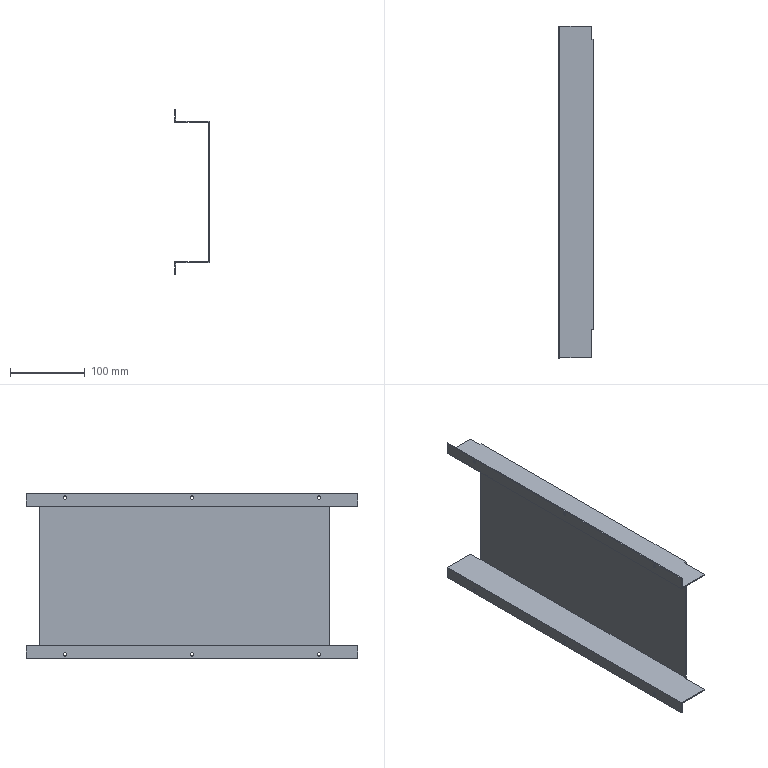Part | SolidWorks | features BaseBody 1 | 1 solid | 34 faces | box 46.5 x 444 x 220 mm | volume 190195 mm3 | plane 22 | cylinder 12 | commonest cylinder face diameters 4.4 x12
STEP:
#1=CARTESIAN_POINT('',(900.946,-4005.973,1042.771));
#2=VERTEX_POINT('',#1);
#3=CARTESIAN_POINT('',(900.946,-4005.973,1047.171));
#4=VERTEX_POINT('',#3);
#5=CARTESIAN_POINT('',(900.946,-4005.973,1044.971));
#6=DIRECTION('',(-1.,0.,0.));
#7=DIRECTION('',(0.,0.,1.));
#8=AXIS2_PLACEMENT_3D('',#5,#6,#7);
#9=CIRCLE('',#8,2.2);
#10=EDGE_CURVE('',#2,#4,#9,.T.);
#11=ORIENTED_EDGE('',*,*,#10,.F.);
#12=CARTESIAN_POINT('',(899.446,-4005.973,1042.771));
#13=VERTEX_POINT('',#12);
#14=CARTESIAN_POINT('',(897.509,-4005.973,1042.771));
#15=DIRECTION('',(-1.,0.,0.));
#16=VECTOR('',#15,1000.);
#17=LINE('',#14,#16);
#18=EDGE_CURVE('',#2,#13,#17,.T.);
#19=ORIENTED_EDGE('',*,*,#18,.T.);
#20=CARTESIAN_POINT('',(899.446,-4005.973,1047.171));
#21=VERTEX_POINT('',#20);
#22=CARTESIAN_POINT('',(899.446,-4005.973,1044.971));
#23=DIRECTION('',(1.,0.,0.));
#24=DIRECTION('',(0.,0.,1.));
#25=AXIS2_PLACEMENT_3D('',#22,#23,#24);
#26=CIRCLE('',#25,2.2);
#27=EDGE_CURVE('',#21,#13,#26,.T.);
#28=ORIENTED_EDGE('',*,*,#27,.F.);
#29=CARTESIAN_POINT('',(897.509,-4005.973,1047.171));
#30=DIRECTION('',(-1.,0.,0.));
#31=VECTOR('',#30,1000.);
#32=LINE('',#29,#31);
#33=EDGE_CURVE('',#4,#21,#32,.T.);
#34=ORIENTED_EDGE('',*,*,#33,.F.);
#35=EDGE_LOOP('',(#11,#19,#28,#34));
#36=FACE_OUTER_BOUND('',#35,.T.);
#37=CARTESIAN_POINT('',(897.509,-4005.973,1044.971));
#38=DIRECTION('',(-1.,0.,0.));
#39=DIRECTION('',(0.,0.,1.));
#40=AXIS2_PLACEMENT_3D('',#37,#38,#39);
#41=CYLINDRICAL_SURFACE('',#40,2.2);
#42=ADVANCED_FACE('',(#36),#41,.F.);
#43=CARTESIAN_POINT('',(900.946,-4345.973,1042.771));
#44=VERTEX_POINT('',#43);
#45=CARTESIAN_POINT('',(900.946,-4345.973,1047.171));
#46=VERTEX_POINT('',#45);
#47=CARTESIAN_POINT('',(900.946,-4345.973,1044.971));
#48=DIRECTION('',(-1.,0.,0.));
#49=DIRECTION('',(0.,0.,1.));
#50=AXIS2_PLACEMENT_3D('',#47,#48,#49);
#51=CIRCLE('',#50,2.2);
#52=EDGE_CURVE('',#44,#46,#51,.T.);
#53=ORIENTED_EDGE('',*,*,#52,.F.);
#54=CARTESIAN_POINT('',(899.446,-4345.973,1042.771));
#55=VERTEX_POINT('',#54);
#56=CARTESIAN_POINT('',(897.509,-4345.973,1042.771));
#57=DIRECTION('',(-1.,0.,0.));
#58=VECTOR('',#57,1000.);
#59=LINE('',#56,#58);
#60=EDGE_CURVE('',#44,#55,#59,.T.);
#61=ORIENTED_EDGE('',*,*,#60,.T.);
#62=CARTESIAN_POINT('',(899.446,-4345.973,1047.171));
#63=VERTEX_POINT('',#62);
#64=CARTESIAN_POINT('',(899.446,-4345.973,1044.971));
#65=DIRECTION('',(1.,0.,0.));
#66=DIRECTION('',(0.,0.,1.));
#67=AXIS2_PLACEMENT_3D('',#64,#65,#66);
#68=CIRCLE('',#67,2.2);
#69=EDGE_CURVE('',#63,#55,#68,.T.);
#70=ORIENTED_EDGE('',*,*,#69,.F.);
#71=CARTESIAN_POINT('',(897.509,-4345.973,1047.171));
#72=DIRECTION('',(-1.,0.,0.));
#73=VECTOR('',#72,1000.);
#74=LINE('',#71,#73);
#75=EDGE_CURVE('',#46,#63,#74,.T.);
#76=ORIENTED_EDGE('',*,*,#75,.F.);
#77=EDGE_LOOP('',(#53,#61,#70,#76));
#78=FACE_OUTER_BOUND('',#77,.T.);
#79=CARTESIAN_POINT('',(897.509,-4345.973,1044.971));
#80=DIRECTION('',(-1.,0.,0.));
#81=DIRECTION('',(0.,0.,1.));
#82=AXIS2_PLACEMENT_3D('',#79,#80,#81);
#83=CYLINDRICAL_SURFACE('',#82,2.2);
#84=ADVANCED_FACE('',(#78),#83,.F.);
#85=CARTESIAN_POINT('',(900.946,-4175.973,1042.771));
#86=VERTEX_POINT('',#85);
#87=CARTESIAN_POINT('',(900.946,-4175.973,1047.171));
#88=VERTEX_POINT('',#87);
#89=CARTESIAN_POINT('',(900.946,-4175.973,1044.971));
#90=DIRECTION('',(-1.,0.,0.));
#91=DIRECTION('',(0.,0.,1.));
#92=AXIS2_PLACEMENT_3D('',#89,#90,#91);
#93=CIRCLE('',#92,2.2);
#94=EDGE_CURVE('',#86,#88,#93,.T.);
#95=ORIENTED_EDGE('',*,*,#94,.F.);
#96=CARTESIAN_POINT('',(899.446,-4175.973,1042.771));
#97=VERTEX_POINT('',#96);
#98=CARTESIAN_POINT('',(897.509,-4175.973,1042.771));
#99=DIRECTION('',(-1.,0.,0.));
#100=VECTOR('',#99,1000.);
#101=LINE('',#98,#100);
#102=EDGE_CURVE('',#86,#97,#101,.T.);
#103=ORIENTED_EDGE('',*,*,#102,.T.);
#104=CARTESIAN_POINT('',(899.446,-4175.973,1047.171));
#105=VERTEX_POINT('',#104);
#106=CARTESIAN_POINT('',(899.446,-4175.973,1044.971));
#107=DIRECTION('',(1.,0.,0.));
#108=DIRECTION('',(0.,0.,1.));
#109=AXIS2_PLACEMENT_3D('',#106,#107,#108);
#110=CIRCLE('',#109,2.2);
#111=EDGE_CURVE('',#105,#97,#110,.T.);
#112=ORIENTED_EDGE('',*,*,#111,.F.);
#113=CARTESIAN_POINT('',(897.509,-4175.973,1047.171));
#114=DIRECTION('',(-1.,0.,0.));
#115=VECTOR('',#114,1000.);
#116=LINE('',#113,#115);
#117=EDGE_CURVE('',#88,#105,#116,.T.);
#118=ORIENTED_EDGE('',*,*,#117,.F.);
#119=EDGE_LOOP('',(#95,#103,#112,#118));
#120=FACE_OUTER_BOUND('',#119,.T.);
#121=CARTESIAN_POINT('',(897.509,-4175.973,1044.971));
#122=DIRECTION('',(-1.,0.,0.));
#123=DIRECTION('',(0.,0.,1.));
#124=AXIS2_PLACEMENT_3D('',#121,#122,#123);
#125=CYLINDRICAL_SURFACE('',#124,2.2);
#126=ADVANCED_FACE('',(#120),#125,.F.);
#127=CARTESIAN_POINT('',(899.446,-4175.973,837.171));
#128=VERTEX_POINT('',#127);
#129=CARTESIAN_POINT('',(899.446,-4175.973,832.771));
#130=VERTEX_POINT('',#129);
#131=CARTESIAN_POINT('',(899.446,-4175.973,834.971));
#132=DIRECTION('',(1.,0.,0.));
#133=DIRECTION('',(0.,0.,-1.));
#134=AXIS2_PLACEMENT_3D('',#131,#132,#133);
#135=CIRCLE('',#134,2.2);
#136=EDGE_CURVE('',#128,#130,#135,.T.);
#137=ORIENTED_EDGE('',*,*,#136,.F.);
#138=CARTESIAN_POINT('',(900.946,-4175.973,837.171));
#139=VERTEX_POINT('',#138);
#140=CARTESIAN_POINT('',(897.509,-4175.973,837.171));
#141=DIRECTION('',(1.,0.,0.));
#142=VECTOR('',#141,1000.);
#143=LINE('',#140,#142);
#144=EDGE_CURVE('',#128,#139,#143,.T.);
#145=ORIENTED_EDGE('',*,*,#144,.T.);
#146=CARTESIAN_POINT('',(900.946,-4175.973,832.771));
#147=VERTEX_POINT('',#146);
#148=CARTESIAN_POINT('',(900.946,-4175.973,834.971));
#149=DIRECTION('',(-1.,0.,0.));
#150=DIRECTION('',(0.,0.,-1.));
#151=AXIS2_PLACEMENT_3D('',#148,#149,#150);
#152=CIRCLE('',#151,2.2);
#153=EDGE_CURVE('',#147,#139,#152,.T.);
#154=ORIENTED_EDGE('',*,*,#153,.F.);
#155=CARTESIAN_POINT('',(897.509,-4175.973,832.771));
#156=DIRECTION('',(1.,0.,0.));
#157=VECTOR('',#156,1000.);
#158=LINE('',#155,#157);
#159=EDGE_CURVE('',#130,#147,#158,.T.);
#160=ORIENTED_EDGE('',*,*,#159,.F.);
#161=EDGE_LOOP('',(#137,#145,#154,#160));
#162=FACE_OUTER_BOUND('',#161,.T.);
#163=CARTESIAN_POINT('',(897.509,-4175.973,834.971));
#164=DIRECTION('',(1.,0.,0.));
#165=DIRECTION('',(0.,0.,-1.));
#166=AXIS2_PLACEMENT_3D('',#163,#164,#165);
#167=CYLINDRICAL_SURFACE('',#166,2.2);
#168=ADVANCED_FACE('',(#162),#167,.F.);
#169=CARTESIAN_POINT('',(899.446,-4345.973,837.171));
#170=VERTEX_POINT('',#169);
#171=CARTESIAN_POINT('',(899.446,-4345.973,832.771));
#172=VERTEX_POINT('',#171);
#173=CARTESIAN_POINT('',(899.446,-4345.973,834.971));
#174=DIRECTION('',(1.,0.,0.));
#175=DIRECTION('',(0.,0.,-1.));
#176=AXIS2_PLACEMENT_3D('',#173,#174,#175);
#177=CIRCLE('',#176,2.2);
#178=EDGE_CURVE('',#170,#172,#177,.T.);
#179=ORIENTED_EDGE('',*,*,#178,.F.);
#180=CARTESIAN_POINT('',(900.946,-4345.973,837.171));
#181=VERTEX_POINT('',#180);
#182=CARTESIAN_POINT('',(897.509,-4345.973,837.171));
#183=DIRECTION('',(1.,0.,0.));
#184=VECTOR('',#183,1000.);
#185=LINE('',#182,#184);
#186=EDGE_CURVE('',#170,#181,#185,.T.);
#187=ORIENTED_EDGE('',*,*,#186,.T.);
#188=CARTESIAN_POINT('',(900.946,-4345.973,832.771));
#189=VERTEX_POINT('',#188);
#190=CARTESIAN_POINT('',(900.946,-4345.973,834.971));
#191=DIRECTION('',(-1.,0.,0.));
#192=DIRECTION('',(0.,0.,-1.));
#193=AXIS2_PLACEMENT_3D('',#190,#191,#192);
#194=CIRCLE('',#193,2.2);
#195=EDGE_CURVE('',#189,#181,#194,.T.);
#196=ORIENTED_EDGE('',*,*,#195,.F.);
#197=CARTESIAN_POINT('',(897.509,-4345.973,832.771));
#198=DIRECTION('',(1.,0.,0.));
#199=VECTOR('',#198,1000.);
#200=LINE('',#197,#199);
#201=EDGE_CURVE('',#172,#189,#200,.T.);
#202=ORIENTED_EDGE('',*,*,#201,.F.);
#203=EDGE_LOOP('',(#179,#187,#196,#202));
#204=FACE_OUTER_BOUND('',#203,.T.);
#205=CARTESIAN_POINT('',(897.509,-4345.973,834.971));
#206=DIRECTION('',(1.,0.,0.));
#207=DIRECTION('',(0.,0.,-1.));
#208=AXIS2_PLACEMENT_3D('',#205,#206,#207);
#209=CYLINDRICAL_SURFACE('',#208,2.2);
#210=ADVANCED_FACE('',(#204),#209,.F.);
#211=CARTESIAN_POINT('',(899.446,-4005.973,837.171));
#212=VERTEX_POINT('',#211);
#213=CARTESIAN_POINT('',(899.446,-4005.973,832.771));
#214=VERTEX_POINT('',#213);
#215=CARTESIAN_POINT('',(899.446,-4005.973,834.971));
#216=DIRECTION('',(1.,0.,0.));
#217=DIRECTION('',(0.,0.,-1.));
#218=AXIS2_PLACEMENT_3D('',#215,#216,#217);
#219=CIRCLE('',#218,2.2);
#220=EDGE_CURVE('',#212,#214,#219,.T.);
#221=ORIENTED_EDGE('',*,*,#220,.F.);
#222=CARTESIAN_POINT('',(900.946,-4005.973,837.171));
#223=VERTEX_POINT('',#222);
#224=CARTESIAN_POINT('',(897.509,-4005.973,837.171));
#225=DIRECTION('',(1.,0.,0.));
#226=VECTOR('',#225,1000.);
#227=LINE('',#224,#226);
#228=EDGE_CURVE('',#212,#223,#227,.T.);
#229=ORIENTED_EDGE('',*,*,#228,.T.);
#230=CARTESIAN_POINT('',(900.946,-4005.973,832.771));
#231=VERTEX_POINT('',#230);
#232=CARTESIAN_POINT('',(900.946,-4005.973,834.971));
#233=DIRECTION('',(-1.,0.,0.));
#234=DIRECTION('',(0.,0.,-1.));
#235=AXIS2_PLACEMENT_3D('',#232,#233,#234);
#236=CIRCLE('',#235,2.2);
#237=EDGE_CURVE('',#231,#223,#236,.T.);
#238=ORIENTED_EDGE('',*,*,#237,.F.);
#239=CARTESIAN_POINT('',(897.509,-4005.973,832.771));
#240=DIRECTION('',(1.,0.,0.));
#241=VECTOR('',#240,1000.);
#242=LINE('',#239,#241);
#243=EDGE_CURVE('',#214,#231,#242,.T.);
#244=ORIENTED_EDGE('',*,*,#243,.F.);
#245=EDGE_LOOP('',(#221,#229,#238,#244));
#246=FACE_OUTER_BOUND('',#245,.T.);
#247=CARTESIAN_POINT('',(897.509,-4005.973,834.971));
#248=DIRECTION('',(1.,0.,0.));
#249=DIRECTION('',(0.,0.,-1.));
#250=AXIS2_PLACEMENT_3D('',#247,#248,#249);
#251=CYLINDRICAL_SURFACE('',#250,2.2);
#252=ADVANCED_FACE('',(#246),#251,.F.);
#253=CARTESIAN_POINT('',(945.946,-3971.973,844.971));
#254=VERTEX_POINT('',#253);
#255=CARTESIAN_POINT('',(945.946,-3971.973,1034.971));
#256=VERTEX_POINT('',#255);
#257=CARTESIAN_POINT('',(945.946,-3971.973,1014.971));
#258=DIRECTION('',(0.,0.,1.));
#259=VECTOR('',#258,1000.);
#260=LINE('',#257,#259);
#261=EDGE_CURVE('',#254,#256,#260,.T.);
#262=ORIENTED_EDGE('',*,*,#261,.T.);
#263=CARTESIAN_POINT('',(945.946,-4359.973,1034.971));
#264=VERTEX_POINT('',#263);
#265=CARTESIAN_POINT('',(945.946,-3953.973,1034.971));
#266=DIRECTION('',(0.,-1.,0.));
#267=VECTOR('',#266,1000.);
#268=LINE('',#265,#267);
#269=EDGE_CURVE('',#256,#264,#268,.T.);
#270=ORIENTED_EDGE('',*,*,#269,.T.);
#271=CARTESIAN_POINT('',(945.946,-4359.973,844.971));
#272=VERTEX_POINT('',#271);
#273=CARTESIAN_POINT('',(945.946,-4359.973,1014.971));
#274=DIRECTION('',(0.,0.,-1.));
#275=VECTOR('',#274,1000.);
#276=LINE('',#273,#275);
#277=EDGE_CURVE('',#264,#272,#276,.T.);
#278=ORIENTED_EDGE('',*,*,#277,.T.);
#279=CARTESIAN_POINT('',(945.946,-3953.973,844.971));
#280=DIRECTION('',(0.,1.,0.));
#281=VECTOR('',#280,1000.);
#282=LINE('',#279,#281);
#283=EDGE_CURVE('',#272,#254,#282,.T.);
#284=ORIENTED_EDGE('',*,*,#283,.T.);
#285=EDGE_LOOP('',(#262,#270,#278,#284));
#286=FACE_OUTER_BOUND('',#285,.T.);
#287=CARTESIAN_POINT('',(945.946,-3953.973,1014.971));
#288=DIRECTION('',(1.,0.,0.));
#289=DIRECTION('',(0.,0.,-1.));
#290=AXIS2_PLACEMENT_3D('',#287,#288,#289);
#291=PLANE('',#290);
#292=ADVANCED_FACE('',(#286),#291,.T.);
#293=CARTESIAN_POINT('',(900.946,-4397.973,1034.971));
#294=VERTEX_POINT('',#293);
#295=CARTESIAN_POINT('',(943.446,-4397.973,1034.971));
#296=VERTEX_POINT('',#295);
#297=CARTESIAN_POINT('',(900.946,-4397.973,1034.971));
#298=DIRECTION('',(1.,0.,0.));
#299=VECTOR('',#298,1000.);
#300=LINE('',#297,#299);
#301=EDGE_CURVE('',#294,#296,#300,.T.);
#302=ORIENTED_EDGE('',*,*,#301,.T.);
#303=CARTESIAN_POINT('',(943.446,-4359.973,1034.971));
#304=VERTEX_POINT('',#303);
#305=CARTESIAN_POINT('',(943.446,-3953.973,1034.971));
#306=DIRECTION('',(0.,1.,0.));
#307=VECTOR('',#306,1000.);
#308=LINE('',#305,#307);
#309=EDGE_CURVE('',#296,#304,#308,.T.);
#310=ORIENTED_EDGE('',*,*,#309,.T.);
#311=CARTESIAN_POINT('',(900.946,-4359.973,1034.971));
#312=DIRECTION('',(1.,0.,0.));
#313=VECTOR('',#312,1000.);
#314=LINE('',#311,#313);
#315=EDGE_CURVE('',#304,#264,#314,.T.);
#316=ORIENTED_EDGE('',*,*,#315,.T.);
#317=ORIENTED_EDGE('',*,*,#269,.F.);
#318=CARTESIAN_POINT('',(943.446,-3971.973,1034.971));
#319=VERTEX_POINT('',#318);
#320=CARTESIAN_POINT('',(900.946,-3971.973,1034.971));
#321=DIRECTION('',(-1.,0.,0.));
#322=VECTOR('',#321,1000.);
#323=LINE('',#320,#322);
#324=EDGE_CURVE('',#256,#319,#323,.T.);
#325=ORIENTED_EDGE('',*,*,#324,.T.);
#326=CARTESIAN_POINT('',(943.446,-3953.973,1034.971));
#327=VERTEX_POINT('',#326);
#328=CARTESIAN_POINT('',(943.446,-3953.973,1034.971));
#329=DIRECTION('',(0.,1.,0.));
#330=VECTOR('',#329,1000.);
#331=LINE('',#328,#330);
#332=EDGE_CURVE('',#319,#327,#331,.T.);
#333=ORIENTED_EDGE('',*,*,#332,.T.);
#334=CARTESIAN_POINT('',(900.946,-3953.973,1034.971));
#335=VERTEX_POINT('',#334);
#336=CARTESIAN_POINT('',(900.946,-3953.973,1034.971));
#337=DIRECTION('',(-1.,0.,0.));
#338=VECTOR('',#337,1000.);
#339=LINE('',#336,#338);
#340=EDGE_CURVE('',#327,#335,#339,.T.);
#341=ORIENTED_EDGE('',*,*,#340,.T.);
#342=CARTESIAN_POINT('',(900.946,-3953.973,1034.971));
#343=DIRECTION('',(0.,-1.,0.));
#344=VECTOR('',#343,1000.);
#345=LINE('',#342,#344);
#346=EDGE_CURVE('',#335,#294,#345,.T.);
#347=ORIENTED_EDGE('',*,*,#346,.T.);
#348=EDGE_LOOP('',(#302,#310,#316,#317,#325,#333,#341,#347));
#349=FACE_OUTER_BOUND('',#348,.T.);
#350=CARTESIAN_POINT('',(900.946,-3953.973,1034.971));
#351=DIRECTION('',(0.,0.,1.));
#352=DIRECTION('',(0.,-1.,0.));
#353=AXIS2_PLACEMENT_3D('',#350,#351,#352);
#354=PLANE('',#353);
#355=ADVANCED_FACE('',(#349),#354,.T.);
#356=CARTESIAN_POINT('',(943.446,-3971.973,844.971));
#357=VERTEX_POINT('',#356);
#358=CARTESIAN_POINT('',(943.446,-3971.973,846.471));
#359=VERTEX_POINT('',#358);
#360=CARTESIAN_POINT('',(943.446,-3971.973,1259.971));
#361=DIRECTION('',(0.,0.,1.));
#362=VECTOR('',#361,1000.);
#363=LINE('',#360,#362);
#364=EDGE_CURVE('',#357,#359,#363,.T.);
#365=ORIENTED_EDGE('',*,*,#364,.T.);
#366=CARTESIAN_POINT('',(944.446,-3971.973,846.471));
#367=VERTEX_POINT('',#366);
#368=CARTESIAN_POINT('',(899.446,-3971.973,846.471));
#369=DIRECTION('',(-1.,0.,0.));
#370=VECTOR('',#369,1000.);
#371=LINE('',#368,#370);
#372=EDGE_CURVE('',#367,#359,#371,.T.);
#373=ORIENTED_EDGE('',*,*,#372,.F.);
#374=CARTESIAN_POINT('',(944.446,-3971.973,1033.471));
#375=VERTEX_POINT('',#374);
#376=CARTESIAN_POINT('',(944.446,-3971.973,2329.971));
#377=DIRECTION('',(0.,0.,-1.));
#378=VECTOR('',#377,1000.);
#379=LINE('',#376,#378);
#380=EDGE_CURVE('',#375,#367,#379,.T.);
#381=ORIENTED_EDGE('',*,*,#380,.F.);
#382=CARTESIAN_POINT('',(943.446,-3971.973,1033.471));
#383=VERTEX_POINT('',#382);
#384=CARTESIAN_POINT('',(944.446,-3971.973,1033.471));
#385=DIRECTION('',(1.,0.,0.));
#386=VECTOR('',#385,1000.);
#387=LINE('',#384,#386);
#388=EDGE_CURVE('',#383,#375,#387,.T.);
#389=ORIENTED_EDGE('',*,*,#388,.F.);
#390=CARTESIAN_POINT('',(943.446,-3971.973,2329.971));
#391=DIRECTION('',(0.,0.,-1.));
#392=VECTOR('',#391,1000.);
#393=LINE('',#390,#392);
#394=EDGE_CURVE('',#319,#383,#393,.T.);
#395=ORIENTED_EDGE('',*,*,#394,.F.);
#396=ORIENTED_EDGE('',*,*,#324,.F.);
#397=ORIENTED_EDGE('',*,*,#261,.F.);
#398=CARTESIAN_POINT('',(944.446,-3971.973,844.971));
#399=DIRECTION('',(1.,0.,0.));
#400=VECTOR('',#399,1000.);
#401=LINE('',#398,#400);
#402=EDGE_CURVE('',#357,#254,#401,.T.);
#403=ORIENTED_EDGE('',*,*,#402,.F.);
#404=EDGE_LOOP('',(#365,#373,#381,#389,#395,#396,#397,#403));
#405=FACE_OUTER_BOUND('',#404,.T.);
#406=CARTESIAN_POINT('',(944.446,-3971.973,2329.971));
#407=DIRECTION('',(0.,-1.,0.));
#408=DIRECTION('',(0.,0.,-1.));
#409=AXIS2_PLACEMENT_3D('',#406,#407,#408);
#410=PLANE('',#409);
#411=ADVANCED_FACE('',(#405),#410,.F.);
#412=ORIENTED_EDGE('',*,*,#402,.T.);
#413=ORIENTED_EDGE('',*,*,#283,.F.);
#414=CARTESIAN_POINT('',(943.446,-4359.973,844.971));
#415=VERTEX_POINT('',#414);
#416=CARTESIAN_POINT('',(945.946,-4359.973,844.971));
#417=DIRECTION('',(-1.,0.,0.));
#418=VECTOR('',#417,1000.);
#419=LINE('',#416,#418);
#420=EDGE_CURVE('',#272,#415,#419,.T.);
#421=ORIENTED_EDGE('',*,*,#420,.T.);
#422=CARTESIAN_POINT('',(943.446,-4397.973,844.971));
#423=VERTEX_POINT('',#422);
#424=CARTESIAN_POINT('',(943.446,-3953.973,844.971));
#425=DIRECTION('',(0.,-1.,0.));
#426=VECTOR('',#425,1000.);
#427=LINE('',#424,#426);
#428=EDGE_CURVE('',#415,#423,#427,.T.);
#429=ORIENTED_EDGE('',*,*,#428,.T.);
#430=CARTESIAN_POINT('',(900.946,-4397.973,844.971));
#431=VERTEX_POINT('',#430);
#432=CARTESIAN_POINT('',(945.946,-4397.973,844.971));
#433=DIRECTION('',(-1.,0.,0.));
#434=VECTOR('',#433,1000.);
#435=LINE('',#432,#434);
#436=EDGE_CURVE('',#423,#431,#435,.T.);
#437=ORIENTED_EDGE('',*,*,#436,.T.);
#438=CARTESIAN_POINT('',(900.946,-3953.973,844.971));
#439=VERTEX_POINT('',#438);
#440=CARTESIAN_POINT('',(900.946,-3953.973,844.971));
#441=DIRECTION('',(0.,1.,0.));
#442=VECTOR('',#441,1000.);
#443=LINE('',#440,#442);
#444=EDGE_CURVE('',#431,#439,#443,.T.);
#445=ORIENTED_EDGE('',*,*,#444,.T.);
#446=CARTESIAN_POINT('',(943.446,-3953.973,844.971));
#447=VERTEX_POINT('',#446);
#448=CARTESIAN_POINT('',(945.946,-3953.973,844.971));
#449=DIRECTION('',(1.,0.,0.));
#450=VECTOR('',#449,1000.);
#451=LINE('',#448,#450);
#452=EDGE_CURVE('',#439,#447,#451,.T.);
#453=ORIENTED_EDGE('',*,*,#452,.T.);
#454=CARTESIAN_POINT('',(943.446,-3953.973,844.971));
#455=DIRECTION('',(0.,-1.,0.));
#456=VECTOR('',#455,1000.);
#457=LINE('',#454,#456);
#458=EDGE_CURVE('',#447,#357,#457,.T.);
#459=ORIENTED_EDGE('',*,*,#458,.T.);
#460=EDGE_LOOP('',(#412,#413,#421,#429,#437,#445,#453,#459));
#461=FACE_OUTER_BOUND('',#460,.T.);
#462=CARTESIAN_POINT('',(945.946,-3953.973,844.971));
#463=DIRECTION('',(0.,0.,-1.));
#464=DIRECTION('',(-1.,0.,0.));
#465=AXIS2_PLACEMENT_3D('',#462,#463,#464);
#466=PLANE('',#465);
#467=ADVANCED_FACE('',(#461),#466,.T.);
#468=ORIENTED_EDGE('',*,*,#277,.F.);
#469=ORIENTED_EDGE('',*,*,#315,.F.);
#470=CARTESIAN_POINT('',(943.446,-4359.973,1033.471));
#471=VERTEX_POINT('',#470);
#472=CARTESIAN_POINT('',(943.446,-4359.973,454.971));
#473=DIRECTION('',(0.,0.,1.));
#474=VECTOR('',#473,1000.);
#475=LINE('',#472,#474);
#476=EDGE_CURVE('',#471,#304,#475,.T.);
#477=ORIENTED_EDGE('',*,*,#476,.F.);
#478=CARTESIAN_POINT('',(944.446,-4359.973,1033.471));
#479=VERTEX_POINT('',#478);
#480=CARTESIAN_POINT('',(944.446,-4359.973,1033.471));
#481=DIRECTION('',(-1.,0.,0.));
#482=VECTOR('',#481,1000.);
#483=LINE('',#480,#482);
#484=EDGE_CURVE('',#479,#471,#483,.T.);
#485=ORIENTED_EDGE('',*,*,#484,.F.);
#486=CARTESIAN_POINT('',(944.446,-4359.973,846.471));
#487=VERTEX_POINT('',#486);
#488=CARTESIAN_POINT('',(944.446,-4359.973,454.971));
#489=DIRECTION('',(0.,0.,1.));
#490=VECTOR('',#489,1000.);
#491=LINE('',#488,#490);
#492=EDGE_CURVE('',#487,#479,#491,.T.);
#493=ORIENTED_EDGE('',*,*,#492,.F.);
#494=CARTESIAN_POINT('',(943.446,-4359.973,846.471));
#495=VERTEX_POINT('',#494);
#496=CARTESIAN_POINT('',(899.446,-4359.973,846.471));
#497=DIRECTION('',(1.,0.,0.));
#498=VECTOR('',#497,1000.);
#499=LINE('',#496,#498);
#500=EDGE_CURVE('',#495,#487,#499,.T.);
#501=ORIENTED_EDGE('',*,*,#500,.F.);
#502=CARTESIAN_POINT('',(943.446,-4359.973,454.971));
#503=DIRECTION('',(0.,0.,1.));
#504=VECTOR('',#503,1000.);
#505=LINE('',#502,#504);
#506=EDGE_CURVE('',#415,#495,#505,.T.);
#507=ORIENTED_EDGE('',*,*,#506,.F.);
#508=ORIENTED_EDGE('',*,*,#420,.F.);
#509=EDGE_LOOP('',(#468,#469,#477,#485,#493,#501,#507,#508));
#510=FACE_OUTER_BOUND('',#509,.T.);
#511=CARTESIAN_POINT('',(946.946,-4359.973,454.971));
#512=DIRECTION('',(0.,1.,0.));
#513=DIRECTION('',(0.,0.,1.));
#514=AXIS2_PLACEMENT_3D('',#511,#512,#513);
#515=PLANE('',#514);
#516=ADVANCED_FACE('',(#510),#515,.F.);
#517=CARTESIAN_POINT('',(943.446,-4397.973,1033.471));
#518=VERTEX_POINT('',#517);
#519=CARTESIAN_POINT('',(943.446,-4397.973,454.971));
#520=DIRECTION('',(0.,0.,1.));
#521=VECTOR('',#520,1000.);
#522=LINE('',#519,#521);
#523=EDGE_CURVE('',#518,#296,#522,.T.);
#524=ORIENTED_EDGE('',*,*,#523,.F.);
#525=CARTESIAN_POINT('',(943.446,-4360.973,1033.471));
#526=DIRECTION('',(0.,-1.,0.));
#527=VECTOR('',#526,1000.);
#528=LINE('',#525,#527);
#529=EDGE_CURVE('',#471,#518,#528,.T.);
#530=ORIENTED_EDGE('',*,*,#529,.F.);
#531=ORIENTED_EDGE('',*,*,#476,.T.);
#532=ORIENTED_EDGE('',*,*,#309,.F.);
#533=EDGE_LOOP('',(#524,#530,#531,#532));
#534=FACE_OUTER_BOUND('',#533,.T.);
#535=CARTESIAN_POINT('',(943.446,-4360.973,454.971));
#536=DIRECTION('',(-1.,0.,0.));
#537=DIRECTION('',(0.,-1.,0.));
#538=AXIS2_PLACEMENT_3D('',#535,#536,#537);
#539=PLANE('',#538);
#540=ADVANCED_FACE('',(#534),#539,.F.);
#541=ORIENTED_EDGE('',*,*,#301,.F.);
#542=CARTESIAN_POINT('',(900.946,-4397.973,1049.971));
#543=VERTEX_POINT('',#542);
#544=CARTESIAN_POINT('',(900.946,-4397.973,949.971));
#545=DIRECTION('',(0.,0.,-1.));
#546=VECTOR('',#545,1000.);
#547=LINE('',#544,#546);
#548=EDGE_CURVE('',#543,#294,#547,.T.);
#549=ORIENTED_EDGE('',*,*,#548,.F.);
#550=CARTESIAN_POINT('',(899.446,-4397.973,1049.971));
#551=VERTEX_POINT('',#550);
#552=CARTESIAN_POINT('',(899.446,-4397.973,1049.971));
#553=DIRECTION('',(1.,0.,0.));
#554=VECTOR('',#553,1000.);
#555=LINE('',#552,#554);
#556=EDGE_CURVE('',#551,#543,#555,.T.);
#557=ORIENTED_EDGE('',*,*,#556,.F.);
#558=CARTESIAN_POINT('',(899.446,-4397.973,1033.471));
#559=VERTEX_POINT('',#558);
#560=CARTESIAN_POINT('',(899.446,-4397.973,949.971));
#561=DIRECTION('',(0.,0.,1.));
#562=VECTOR('',#561,1000.);
#563=LINE('',#560,#562);
#564=EDGE_CURVE('',#559,#551,#563,.T.);
#565=ORIENTED_EDGE('',*,*,#564,.F.);
#566=CARTESIAN_POINT('',(933.154,-4397.973,1033.471));
#567=DIRECTION('',(-1.,0.,0.));
#568=VECTOR('',#567,1000.);
#569=LINE('',#566,#568);
#570=EDGE_CURVE('',#518,#559,#569,.T.);
#571=ORIENTED_EDGE('',*,*,#570,.F.);
#572=ORIENTED_EDGE('',*,*,#523,.T.);
#573=EDGE_LOOP('',(#541,#549,#557,#565,#571,#572));
#574=FACE_OUTER_BOUND('',#573,.T.);
#575=CARTESIAN_POINT('',(933.154,-4397.973,949.971));
#576=DIRECTION('',(0.,1.,0.));
#577=DIRECTION('',(0.,0.,1.));
#578=AXIS2_PLACEMENT_3D('',#575,#576,#577);
#579=PLANE('',#578);
#580=ADVANCED_FACE('',(#574),#579,.F.);
#581=CARTESIAN_POINT('',(900.946,-3953.973,1049.971));
#582=VERTEX_POINT('',#581);
#583=CARTESIAN_POINT('',(900.946,-3953.973,1029.971));
#584=DIRECTION('',(0.,0.,1.));
#585=VECTOR('',#584,1000.);
#586=LINE('',#583,#585);
#587=EDGE_CURVE('',#335,#582,#586,.T.);
#588=ORIENTED_EDGE('',*,*,#587,.T.);
#589=CARTESIAN_POINT('',(900.946,-3953.973,1049.971));
#590=DIRECTION('',(0.,-1.,0.));
#591=VECTOR('',#590,1000.);
#592=LINE('',#589,#591);
#593=EDGE_CURVE('',#582,#543,#592,.T.);
#594=ORIENTED_EDGE('',*,*,#593,.T.);
#595=ORIENTED_EDGE('',*,*,#548,.T.);
#596=ORIENTED_EDGE('',*,*,#346,.F.);
#597=EDGE_LOOP('',(#588,#594,#595,#596));
#598=FACE_OUTER_BOUND('',#597,.T.);
#599=CARTESIAN_POINT('',(900.946,-4005.973,1044.971));
#600=DIRECTION('',(-1.,0.,0.));
#601=DIRECTION('',(0.,0.,1.));
#602=AXIS2_PLACEMENT_3D('',#599,#600,#601);
#603=CIRCLE('',#602,2.2);
#604=EDGE_CURVE('',#4,#2,#603,.T.);
#605=ORIENTED_EDGE('',*,*,#604,.T.);
#606=ORIENTED_EDGE('',*,*,#10,.T.);
#607=EDGE_LOOP('',(#605,#606));
#608=FACE_BOUND('',#607,.T.);
#609=CARTESIAN_POINT('',(900.946,-4345.973,1044.971));
#610=DIRECTION('',(-1.,0.,0.));
#611=DIRECTION('',(0.,0.,1.));
#612=AXIS2_PLACEMENT_3D('',#609,#610,#611);
#613=CIRCLE('',#612,2.2);
#614=EDGE_CURVE('',#46,#44,#613,.T.);
#615=ORIENTED_EDGE('',*,*,#614,.T.);
#616=ORIENTED_EDGE('',*,*,#52,.T.);
#617=EDGE_LOOP('',(#615,#616));
#618=FACE_BOUND('',#617,.T.);
#619=CARTESIAN_POINT('',(900.946,-4175.973,1044.971));
#620=DIRECTION('',(-1.,0.,0.));
#621=DIRECTION('',(0.,0.,1.));
#622=AXIS2_PLACEMENT_3D('',#619,#620,#621);
#623=CIRCLE('',#622,2.2);
#624=EDGE_CURVE('',#88,#86,#623,.T.);
#625=ORIENTED_EDGE('',*,*,#624,.T.);
#626=ORIENTED_EDGE('',*,*,#94,.T.);
#627=EDGE_LOOP('',(#625,#626));
#628=FACE_BOUND('',#627,.T.);
#629=CARTESIAN_POINT('',(900.946,-3953.973,1029.971));
#630=DIRECTION('',(1.,0.,0.));
#631=DIRECTION('',(0.,0.,-1.));
#632=AXIS2_PLACEMENT_3D('',#629,#630,#631);
#633=PLANE('',#632);
#634=ADVANCED_FACE('',(#598,#608,#618,#628),#633,.T.);
#635=ORIENTED_EDGE('',*,*,#587,.F.);
#636=ORIENTED_EDGE('',*,*,#340,.F.);
#637=CARTESIAN_POINT('',(943.446,-3953.973,1033.471));
#638=VERTEX_POINT('',#637);
#639=CARTESIAN_POINT('',(943.446,-3953.973,929.971));
#640=DIRECTION('',(0.,0.,-1.));
#641=VECTOR('',#640,1000.);
#642=LINE('',#639,#641);
#643=EDGE_CURVE('',#327,#638,#642,.T.);
#644=ORIENTED_EDGE('',*,*,#643,.T.);
#645=CARTESIAN_POINT('',(899.446,-3953.973,1033.471));
#646=VERTEX_POINT('',#645);
#647=CARTESIAN_POINT('',(933.154,-3953.973,1033.471));
#648=DIRECTION('',(-1.,0.,0.));
#649=VECTOR('',#648,1000.);
#650=LINE('',#647,#649);
#651=EDGE_CURVE('',#638,#646,#650,.T.);
#652=ORIENTED_EDGE('',*,*,#651,.T.);
#653=CARTESIAN_POINT('',(899.446,-3953.973,1049.971));
#654=VERTEX_POINT('',#653);
#655=CARTESIAN_POINT('',(899.446,-3953.973,929.971));
#656=DIRECTION('',(0.,0.,1.));
#657=VECTOR('',#656,1000.);
#658=LINE('',#655,#657);
#659=EDGE_CURVE('',#646,#654,#658,.T.);
#660=ORIENTED_EDGE('',*,*,#659,.T.);
#661=CARTESIAN_POINT('',(933.154,-3953.973,1049.971));
#662=DIRECTION('',(1.,0.,0.));
#663=VECTOR('',#662,1000.);
#664=LINE('',#661,#663);
#665=EDGE_CURVE('',#654,#582,#664,.T.);
#666=ORIENTED_EDGE('',*,*,#665,.T.);
#667=EDGE_LOOP('',(#635,#636,#644,#652,#660,#666));
#668=FACE_OUTER_BOUND('',#667,.T.);
#669=CARTESIAN_POINT('',(933.154,-3953.973,929.971));
#670=DIRECTION('',(0.,1.,0.));
#671=DIRECTION('',(0.,0.,1.));
#672=AXIS2_PLACEMENT_3D('',#669,#670,#671);
#673=PLANE('',#672);
#674=ADVANCED_FACE('',(#668),#673,.T.);
#675=ORIENTED_EDGE('',*,*,#394,.T.);
#676=CARTESIAN_POINT('',(943.446,-3960.973,1033.471));
#677=DIRECTION('',(0.,-1.,0.));
#678=VECTOR('',#677,1000.);
#679=LINE('',#676,#678);
#680=EDGE_CURVE('',#638,#383,#679,.T.);
#681=ORIENTED_EDGE('',*,*,#680,.F.);
#682=ORIENTED_EDGE('',*,*,#643,.F.);
#683=ORIENTED_EDGE('',*,*,#332,.F.);
#684=EDGE_LOOP('',(#675,#681,#682,#683));
#685=FACE_OUTER_BOUND('',#684,.T.);
#686=CARTESIAN_POINT('',(943.446,-3960.973,1259.971));
#687=DIRECTION('',(-1.,0.,0.));
#688=DIRECTION('',(0.,0.,1.));
#689=AXIS2_PLACEMENT_3D('',#686,#687,#688);
#690=PLANE('',#689);
#691=ADVANCED_FACE('',(#685),#690,.F.);
#692=ORIENTED_EDGE('',*,*,#380,.T.);
#693=CARTESIAN_POINT('',(944.446,-3953.973,846.471));
#694=DIRECTION('',(0.,-1.,0.));
#695=VECTOR('',#694,1000.);
#696=LINE('',#693,#695);
#697=EDGE_CURVE('',#367,#487,#696,.T.);
#698=ORIENTED_EDGE('',*,*,#697,.T.);
#699=ORIENTED_EDGE('',*,*,#492,.T.);
#700=CARTESIAN_POINT('',(944.446,-3953.973,1033.471));
#701=DIRECTION('',(0.,1.,0.));
#702=VECTOR('',#701,1000.);
#703=LINE('',#700,#702);
#704=EDGE_CURVE('',#479,#375,#703,.T.);
#705=ORIENTED_EDGE('',*,*,#704,.T.);
#706=EDGE_LOOP('',(#692,#698,#699,#705));
#707=FACE_OUTER_BOUND('',#706,.T.);
#708=CARTESIAN_POINT('',(944.446,-3953.973,846.471));
#709=DIRECTION('',(-1.,0.,0.));
#710=DIRECTION('',(0.,0.,1.));
#711=AXIS2_PLACEMENT_3D('',#708,#709,#710);
#712=PLANE('',#711);
#713=ADVANCED_FACE('',(#707),#712,.T.);
#714=CARTESIAN_POINT('',(943.446,-3953.973,846.471));
#715=VERTEX_POINT('',#714);
#716=CARTESIAN_POINT('',(943.446,-3953.973,1259.971));
#717=DIRECTION('',(0.,0.,-1.));
#718=VECTOR('',#717,1000.);
#719=LINE('',#716,#718);
#720=EDGE_CURVE('',#715,#447,#719,.T.);
#721=ORIENTED_EDGE('',*,*,#720,.F.);
#722=CARTESIAN_POINT('',(943.446,-3960.973,846.471));
#723=DIRECTION('',(0.,1.,0.));
#724=VECTOR('',#723,1000.);
#725=LINE('',#722,#724);
#726=EDGE_CURVE('',#359,#715,#725,.T.);
#727=ORIENTED_EDGE('',*,*,#726,.F.);
#728=ORIENTED_EDGE('',*,*,#364,.F.);
#729=ORIENTED_EDGE('',*,*,#458,.F.);
#730=EDGE_LOOP('',(#721,#727,#728,#729));
#731=FACE_OUTER_BOUND('',#730,.T.);
#732=CARTESIAN_POINT('',(943.446,-3960.973,1259.971));
#733=DIRECTION('',(-1.,0.,0.));
#734=DIRECTION('',(0.,0.,1.));
#735=AXIS2_PLACEMENT_3D('',#732,#733,#734);
#736=PLANE('',#735);
#737=ADVANCED_FACE('',(#731),#736,.F.);
#738=CARTESIAN_POINT('',(899.446,-3953.973,829.971));
#739=VERTEX_POINT('',#738);
#740=CARTESIAN_POINT('',(899.446,-3953.973,846.471));
#741=VERTEX_POINT('',#740);
#742=CARTESIAN_POINT('',(899.446,-3953.973,929.971));
#743=DIRECTION('',(0.,0.,1.));
#744=VECTOR('',#743,1000.);
#745=LINE('',#742,#744);
#746=EDGE_CURVE('',#739,#741,#745,.T.);
#747=ORIENTED_EDGE('',*,*,#746,.T.);
#748=CARTESIAN_POINT('',(933.154,-3953.973,846.471));
#749=DIRECTION('',(1.,0.,0.));
#750=VECTOR('',#749,1000.);
#751=LINE('',#748,#750);
#752=EDGE_CURVE('',#741,#715,#751,.T.);
#753=ORIENTED_EDGE('',*,*,#752,.T.);
#754=ORIENTED_EDGE('',*,*,#720,.T.);
#755=ORIENTED_EDGE('',*,*,#452,.F.);
#756=CARTESIAN_POINT('',(900.946,-3953.973,829.971));
#757=VERTEX_POINT('',#756);
#758=CARTESIAN_POINT('',(900.946,-3953.973,929.971));
#759=DIRECTION('',(0.,0.,-1.));
#760=VECTOR('',#759,1000.);
#761=LINE('',#758,#760);
#762=EDGE_CURVE('',#439,#757,#761,.T.);
#763=ORIENTED_EDGE('',*,*,#762,.T.);
#764=CARTESIAN_POINT('',(900.946,-3953.973,829.971));
#765=DIRECTION('',(1.,0.,0.));
#766=VECTOR('',#765,1000.);
#767=LINE('',#764,#766);
#768=EDGE_CURVE('',#739,#757,#767,.T.);
#769=ORIENTED_EDGE('',*,*,#768,.F.);
#770=EDGE_LOOP('',(#747,#753,#754,#755,#763,#769));
#771=FACE_OUTER_BOUND('',#770,.T.);
#772=CARTESIAN_POINT('',(933.154,-3953.973,929.971));
#773=DIRECTION('',(0.,1.,0.));
#774=DIRECTION('',(0.,0.,1.));
#775=AXIS2_PLACEMENT_3D('',#772,#773,#774);
#776=PLANE('',#775);
#777=ADVANCED_FACE('',(#771),#776,.T.);
#778=ORIENTED_EDGE('',*,*,#762,.F.);
#779=ORIENTED_EDGE('',*,*,#444,.F.);
#780=CARTESIAN_POINT('',(900.946,-4397.973,829.971));
#781=VERTEX_POINT('',#780);
#782=CARTESIAN_POINT('',(900.946,-4397.973,844.971));
#783=DIRECTION('',(0.,0.,-1.));
#784=VECTOR('',#783,1000.);
#785=LINE('',#782,#784);
#786=EDGE_CURVE('',#431,#781,#785,.T.);
#787=ORIENTED_EDGE('',*,*,#786,.T.);
#788=CARTESIAN_POINT('',(900.946,-3953.973,829.971));
#789=DIRECTION('',(0.,1.,0.));
#790=VECTOR('',#789,1000.);
#791=LINE('',#788,#790);
#792=EDGE_CURVE('',#781,#757,#791,.T.);
#793=ORIENTED_EDGE('',*,*,#792,.T.);
#794=EDGE_LOOP('',(#778,#779,#787,#793));
#795=FACE_OUTER_BOUND('',#794,.T.);
#796=ORIENTED_EDGE('',*,*,#153,.T.);
#797=CARTESIAN_POINT('',(900.946,-4175.973,834.971));
#798=DIRECTION('',(-1.,0.,0.));
#799=DIRECTION('',(0.,0.,-1.));
#800=AXIS2_PLACEMENT_3D('',#797,#798,#799);
#801=CIRCLE('',#800,2.2);
#802=EDGE_CURVE('',#139,#147,#801,.T.);
#803=ORIENTED_EDGE('',*,*,#802,.T.);
#804=EDGE_LOOP('',(#796,#803));
#805=FACE_BOUND('',#804,.T.);
#806=ORIENTED_EDGE('',*,*,#195,.T.);
#807=CARTESIAN_POINT('',(900.946,-4345.973,834.971));
#808=DIRECTION('',(-1.,0.,0.));
#809=DIRECTION('',(0.,0.,-1.));
#810=AXIS2_PLACEMENT_3D('',#807,#808,#809);
#811=CIRCLE('',#810,2.2);
#812=EDGE_CURVE('',#181,#189,#811,.T.);
#813=ORIENTED_EDGE('',*,*,#812,.T.);
#814=EDGE_LOOP('',(#806,#813));
#815=FACE_BOUND('',#814,.T.);
#816=ORIENTED_EDGE('',*,*,#237,.T.);
#817=CARTESIAN_POINT('',(900.946,-4005.973,834.971));
#818=DIRECTION('',(-1.,0.,0.));
#819=DIRECTION('',(0.,0.,-1.));
#820=AXIS2_PLACEMENT_3D('',#817,#818,#819);
#821=CIRCLE('',#820,2.2);
#822=EDGE_CURVE('',#223,#231,#821,.T.);
#823=ORIENTED_EDGE('',*,*,#822,.T.);
#824=EDGE_LOOP('',(#816,#823));
#825=FACE_BOUND('',#824,.T.);
#826=CARTESIAN_POINT('',(900.946,-3953.973,844.971));
#827=DIRECTION('',(1.,0.,0.));
#828=DIRECTION('',(0.,0.,-1.));
#829=AXIS2_PLACEMENT_3D('',#826,#827,#828);
#830=PLANE('',#829);
#831=ADVANCED_FACE('',(#795,#805,#815,#825),#830,.T.);
#832=CARTESIAN_POINT('',(899.446,-4397.973,846.471));
#833=VERTEX_POINT('',#832);
#834=CARTESIAN_POINT('',(943.446,-4397.973,846.471));
#835=VERTEX_POINT('',#834);
#836=CARTESIAN_POINT('',(933.154,-4397.973,846.471));
#837=DIRECTION('',(1.,0.,0.));
#838=VECTOR('',#837,1000.);
#839=LINE('',#836,#838);
#840=EDGE_CURVE('',#833,#835,#839,.T.);
#841=ORIENTED_EDGE('',*,*,#840,.F.);
#842=CARTESIAN_POINT('',(899.446,-4397.973,829.971));
#843=VERTEX_POINT('',#842);
#844=CARTESIAN_POINT('',(899.446,-4397.973,929.971));
#845=DIRECTION('',(0.,0.,1.));
#846=VECTOR('',#845,1000.);
#847=LINE('',#844,#846);
#848=EDGE_CURVE('',#843,#833,#847,.T.);
#849=ORIENTED_EDGE('',*,*,#848,.F.);
#850=CARTESIAN_POINT('',(933.154,-4397.973,829.971));
#851=DIRECTION('',(-1.,0.,0.));
#852=VECTOR('',#851,1000.);
#853=LINE('',#850,#852);
#854=EDGE_CURVE('',#781,#843,#853,.T.);
#855=ORIENTED_EDGE('',*,*,#854,.F.);
#856=ORIENTED_EDGE('',*,*,#786,.F.);
#857=ORIENTED_EDGE('',*,*,#436,.F.);
#858=CARTESIAN_POINT('',(943.446,-4397.973,929.971));
#859=DIRECTION('',(0.,0.,-1.));
#860=VECTOR('',#859,1000.);
#861=LINE('',#858,#860);
#862=EDGE_CURVE('',#835,#423,#861,.T.);
#863=ORIENTED_EDGE('',*,*,#862,.F.);
#864=EDGE_LOOP('',(#841,#849,#855,#856,#857,#863));
#865=FACE_OUTER_BOUND('',#864,.T.);
#866=CARTESIAN_POINT('',(933.154,-4397.973,929.971));
#867=DIRECTION('',(0.,1.,0.));
#868=DIRECTION('',(0.,0.,1.));
#869=AXIS2_PLACEMENT_3D('',#866,#867,#868);
#870=PLANE('',#869);
#871=ADVANCED_FACE('',(#865),#870,.F.);
#872=ORIENTED_EDGE('',*,*,#506,.T.);
#873=CARTESIAN_POINT('',(943.446,-4360.973,846.471));
#874=DIRECTION('',(0.,1.,0.));
#875=VECTOR('',#874,1000.);
#876=LINE('',#873,#875);
#877=EDGE_CURVE('',#835,#495,#876,.T.);
#878=ORIENTED_EDGE('',*,*,#877,.F.);
#879=ORIENTED_EDGE('',*,*,#862,.T.);
#880=ORIENTED_EDGE('',*,*,#428,.F.);
#881=EDGE_LOOP('',(#872,#878,#879,#880));
#882=FACE_OUTER_BOUND('',#881,.T.);
#883=CARTESIAN_POINT('',(943.446,-4360.973,454.971));
#884=DIRECTION('',(-1.,0.,0.));
#885=DIRECTION('',(0.,-1.,0.));
#886=AXIS2_PLACEMENT_3D('',#883,#884,#885);
#887=PLANE('',#886);
#888=ADVANCED_FACE('',(#882),#887,.F.);
#889=ORIENTED_EDGE('',*,*,#484,.T.);
#890=ORIENTED_EDGE('',*,*,#529,.T.);
#891=ORIENTED_EDGE('',*,*,#570,.T.);
#892=CARTESIAN_POINT('',(899.446,-3953.973,1033.471));
#893=DIRECTION('',(0.,1.,0.));
#894=VECTOR('',#893,1000.);
#895=LINE('',#892,#894);
#896=EDGE_CURVE('',#559,#646,#895,.T.);
#897=ORIENTED_EDGE('',*,*,#896,.T.);
#898=ORIENTED_EDGE('',*,*,#651,.F.);
#899=ORIENTED_EDGE('',*,*,#680,.T.);
#900=ORIENTED_EDGE('',*,*,#388,.T.);
#901=ORIENTED_EDGE('',*,*,#704,.F.);
#902=EDGE_LOOP('',(#889,#890,#891,#897,#898,#899,#900,#901));
#903=FACE_OUTER_BOUND('',#902,.T.);
#904=CARTESIAN_POINT('',(944.446,-3953.973,1033.471));
#905=DIRECTION('',(0.,0.,-1.));
#906=DIRECTION('',(-1.,0.,0.));
#907=AXIS2_PLACEMENT_3D('',#904,#905,#906);
#908=PLANE('',#907);
#909=ADVANCED_FACE('',(#903),#908,.T.);
#910=ORIENTED_EDGE('',*,*,#659,.F.);
#911=ORIENTED_EDGE('',*,*,#896,.F.);
#912=ORIENTED_EDGE('',*,*,#564,.T.);
#913=CARTESIAN_POINT('',(899.446,-3953.973,1049.971));
#914=DIRECTION('',(0.,1.,0.));
#915=VECTOR('',#914,1000.);
#916=LINE('',#913,#915);
#917=EDGE_CURVE('',#551,#654,#916,.T.);
#918=ORIENTED_EDGE('',*,*,#917,.T.);
#919=EDGE_LOOP('',(#910,#911,#912,#918));
#920=FACE_OUTER_BOUND('',#919,.T.);
#921=ORIENTED_EDGE('',*,*,#27,.T.);
#922=CARTESIAN_POINT('',(899.446,-4005.973,1044.971));
#923=DIRECTION('',(1.,0.,0.));
#924=DIRECTION('',(0.,0.,1.));
#925=AXIS2_PLACEMENT_3D('',#922,#923,#924);
#926=CIRCLE('',#925,2.2);
#927=EDGE_CURVE('',#13,#21,#926,.T.);
#928=ORIENTED_EDGE('',*,*,#927,.T.);
#929=EDGE_LOOP('',(#921,#928));
#930=FACE_BOUND('',#929,.T.);
#931=ORIENTED_EDGE('',*,*,#69,.T.);
#932=CARTESIAN_POINT('',(899.446,-4345.973,1044.971));
#933=DIRECTION('',(1.,0.,0.));
#934=DIRECTION('',(0.,0.,1.));
#935=AXIS2_PLACEMENT_3D('',#932,#933,#934);
#936=CIRCLE('',#935,2.2);
#937=EDGE_CURVE('',#55,#63,#936,.T.);
#938=ORIENTED_EDGE('',*,*,#937,.T.);
#939=EDGE_LOOP('',(#931,#938));
#940=FACE_BOUND('',#939,.T.);
#941=ORIENTED_EDGE('',*,*,#111,.T.);
#942=CARTESIAN_POINT('',(899.446,-4175.973,1044.971));
#943=DIRECTION('',(1.,0.,0.));
#944=DIRECTION('',(0.,0.,1.));
#945=AXIS2_PLACEMENT_3D('',#942,#943,#944);
#946=CIRCLE('',#945,2.2);
#947=EDGE_CURVE('',#97,#105,#946,.T.);
#948=ORIENTED_EDGE('',*,*,#947,.T.);
#949=EDGE_LOOP('',(#941,#948));
#950=FACE_BOUND('',#949,.T.);
#951=CARTESIAN_POINT('',(899.446,-3953.973,1013.471));
#952=DIRECTION('',(-1.,0.,0.));
#953=DIRECTION('',(0.,0.,1.));
#954=AXIS2_PLACEMENT_3D('',#951,#952,#953);
#955=PLANE('',#954);
#956=ADVANCED_FACE('',(#920,#930,#940,#950),#955,.T.);
#957=ORIENTED_EDGE('',*,*,#665,.F.);
#958=ORIENTED_EDGE('',*,*,#917,.F.);
#959=ORIENTED_EDGE('',*,*,#556,.T.);
#960=ORIENTED_EDGE('',*,*,#593,.F.);
#961=EDGE_LOOP('',(#957,#958,#959,#960));
#962=FACE_OUTER_BOUND('',#961,.T.);
#963=CARTESIAN_POINT('',(899.446,-3953.973,1049.971));
#964=DIRECTION('',(0.,0.,1.));
#965=DIRECTION('',(1.,0.,0.));
#966=AXIS2_PLACEMENT_3D('',#963,#964,#965);
#967=PLANE('',#966);
#968=ADVANCED_FACE('',(#962),#967,.T.);
#969=ORIENTED_EDGE('',*,*,#18,.F.);
#970=ORIENTED_EDGE('',*,*,#604,.F.);
#971=ORIENTED_EDGE('',*,*,#33,.T.);
#972=ORIENTED_EDGE('',*,*,#927,.F.);
#973=EDGE_LOOP('',(#969,#970,#971,#972));
#974=FACE_OUTER_BOUND('',#973,.T.);
#975=CARTESIAN_POINT('',(897.509,-4005.973,1044.971));
#976=DIRECTION('',(-1.,0.,0.));
#977=DIRECTION('',(0.,0.,1.));
#978=AXIS2_PLACEMENT_3D('',#975,#976,#977);
#979=CYLINDRICAL_SURFACE('',#978,2.2);
#980=ADVANCED_FACE('',(#974),#979,.F.);
#981=ORIENTED_EDGE('',*,*,#60,.F.);
#982=ORIENTED_EDGE('',*,*,#614,.F.);
#983=ORIENTED_EDGE('',*,*,#75,.T.);
#984=ORIENTED_EDGE('',*,*,#937,.F.);
#985=EDGE_LOOP('',(#981,#982,#983,#984));
#986=FACE_OUTER_BOUND('',#985,.T.);
#987=CARTESIAN_POINT('',(897.509,-4345.973,1044.971));
#988=DIRECTION('',(-1.,0.,0.));
#989=DIRECTION('',(0.,0.,1.));
#990=AXIS2_PLACEMENT_3D('',#987,#988,#989);
#991=CYLINDRICAL_SURFACE('',#990,2.2);
#992=ADVANCED_FACE('',(#986),#991,.F.);
#993=ORIENTED_EDGE('',*,*,#102,.F.);
#994=ORIENTED_EDGE('',*,*,#624,.F.);
#995=ORIENTED_EDGE('',*,*,#117,.T.);
#996=ORIENTED_EDGE('',*,*,#947,.F.);
#997=EDGE_LOOP('',(#993,#994,#995,#996));
#998=FACE_OUTER_BOUND('',#997,.T.);
#999=CARTESIAN_POINT('',(897.509,-4175.973,1044.971));
#1000=DIRECTION('',(-1.,0.,0.));
#1001=DIRECTION('',(0.,0.,1.));
#1002=AXIS2_PLACEMENT_3D('',#999,#1000,#1001);
#1003=CYLINDRICAL_SURFACE('',#1002,2.2);
#1004=ADVANCED_FACE('',(#998),#1003,.F.);
#1005=ORIENTED_EDGE('',*,*,#752,.F.);
#1006=CARTESIAN_POINT('',(899.446,-3953.973,846.471));
#1007=DIRECTION('',(0.,-1.,0.));
#1008=VECTOR('',#1007,1000.);
#1009=LINE('',#1006,#1008);
#1010=EDGE_CURVE('',#741,#833,#1009,.T.);
#1011=ORIENTED_EDGE('',*,*,#1010,.T.);
#1012=ORIENTED_EDGE('',*,*,#840,.T.);
#1013=ORIENTED_EDGE('',*,*,#877,.T.);
#1014=ORIENTED_EDGE('',*,*,#500,.T.);
#1015=ORIENTED_EDGE('',*,*,#697,.F.);
#1016=ORIENTED_EDGE('',*,*,#372,.T.);
#1017=ORIENTED_EDGE('',*,*,#726,.T.);
#1018=EDGE_LOOP('',(#1005,#1011,#1012,#1013,#1014,#1015,#1016,#1017));
#1019=FACE_OUTER_BOUND('',#1018,.T.);
#1020=CARTESIAN_POINT('',(899.446,-3953.973,846.471));
#1021=DIRECTION('',(0.,0.,1.));
#1022=DIRECTION('',(1.,0.,0.));
#1023=AXIS2_PLACEMENT_3D('',#1020,#1021,#1022);
#1024=PLANE('',#1023);
#1025=ADVANCED_FACE('',(#1019),#1024,.T.);
#1026=ORIENTED_EDGE('',*,*,#746,.F.);
#1027=CARTESIAN_POINT('',(899.446,-3953.973,829.971));
#1028=DIRECTION('',(0.,-1.,0.));
#1029=VECTOR('',#1028,1000.);
#1030=LINE('',#1027,#1029);
#1031=EDGE_CURVE('',#739,#843,#1030,.T.);
#1032=ORIENTED_EDGE('',*,*,#1031,.T.);
#1033=ORIENTED_EDGE('',*,*,#848,.T.);
#1034=ORIENTED_EDGE('',*,*,#1010,.F.);
#1035=EDGE_LOOP('',(#1026,#1032,#1033,#1034));
#1036=FACE_OUTER_BOUND('',#1035,.T.);
#1037=CARTESIAN_POINT('',(899.446,-4175.973,834.971));
#1038=DIRECTION('',(1.,0.,0.));
#1039=DIRECTION('',(0.,0.,-1.));
#1040=AXIS2_PLACEMENT_3D('',#1037,#1038,#1039);
#1041=CIRCLE('',#1040,2.2);
#1042=EDGE_CURVE('',#130,#128,#1041,.T.);
#1043=ORIENTED_EDGE('',*,*,#1042,.T.);
#1044=ORIENTED_EDGE('',*,*,#136,.T.);
#1045=EDGE_LOOP('',(#1043,#1044));
#1046=FACE_BOUND('',#1045,.T.);
#1047=CARTESIAN_POINT('',(899.446,-4345.973,834.971));
#1048=DIRECTION('',(1.,0.,0.));
#1049=DIRECTION('',(0.,0.,-1.));
#1050=AXIS2_PLACEMENT_3D('',#1047,#1048,#1049);
#1051=CIRCLE('',#1050,2.2);
#1052=EDGE_CURVE('',#172,#170,#1051,.T.);
#1053=ORIENTED_EDGE('',*,*,#1052,.T.);
#1054=ORIENTED_EDGE('',*,*,#178,.T.);
#1055=EDGE_LOOP('',(#1053,#1054));
#1056=FACE_BOUND('',#1055,.T.);
#1057=CARTESIAN_POINT('',(899.446,-4005.973,834.971));
#1058=DIRECTION('',(1.,0.,0.));
#1059=DIRECTION('',(0.,0.,-1.));
#1060=AXIS2_PLACEMENT_3D('',#1057,#1058,#1059);
#1061=CIRCLE('',#1060,2.2);
#1062=EDGE_CURVE('',#214,#212,#1061,.T.);
#1063=ORIENTED_EDGE('',*,*,#1062,.T.);
#1064=ORIENTED_EDGE('',*,*,#220,.T.);
#1065=EDGE_LOOP('',(#1063,#1064));
#1066=FACE_BOUND('',#1065,.T.);
#1067=CARTESIAN_POINT('',(899.446,-3953.973,829.971));
#1068=DIRECTION('',(-1.,0.,0.));
#1069=DIRECTION('',(0.,0.,1.));
#1070=AXIS2_PLACEMENT_3D('',#1067,#1068,#1069);
#1071=PLANE('',#1070);
#1072=ADVANCED_FACE('',(#1036,#1046,#1056,#1066),#1071,.T.);
#1073=ORIENTED_EDGE('',*,*,#768,.T.);
#1074=ORIENTED_EDGE('',*,*,#792,.F.);
#1075=ORIENTED_EDGE('',*,*,#854,.T.);
#1076=ORIENTED_EDGE('',*,*,#1031,.F.);
#1077=EDGE_LOOP('',(#1073,#1074,#1075,#1076));
#1078=FACE_OUTER_BOUND('',#1077,.T.);
#1079=CARTESIAN_POINT('',(900.946,-3953.973,829.971));
#1080=DIRECTION('',(0.,0.,-1.));
#1081=DIRECTION('',(-1.,0.,0.));
#1082=AXIS2_PLACEMENT_3D('',#1079,#1080,#1081);
#1083=PLANE('',#1082);
#1084=ADVANCED_FACE('',(#1078),#1083,.T.);
#1085=ORIENTED_EDGE('',*,*,#144,.F.);
#1086=ORIENTED_EDGE('',*,*,#1042,.F.);
#1087=ORIENTED_EDGE('',*,*,#159,.T.);
#1088=ORIENTED_EDGE('',*,*,#802,.F.);
#1089=EDGE_LOOP('',(#1085,#1086,#1087,#1088));
#1090=FACE_OUTER_BOUND('',#1089,.T.);
#1091=CARTESIAN_POINT('',(897.509,-4175.973,834.971));
#1092=DIRECTION('',(1.,0.,0.));
#1093=DIRECTION('',(0.,0.,-1.));
#1094=AXIS2_PLACEMENT_3D('',#1091,#1092,#1093);
#1095=CYLINDRICAL_SURFACE('',#1094,2.2);
#1096=ADVANCED_FACE('',(#1090),#1095,.F.);
#1097=ORIENTED_EDGE('',*,*,#186,.F.);
#1098=ORIENTED_EDGE('',*,*,#1052,.F.);
#1099=ORIENTED_EDGE('',*,*,#201,.T.);
#1100=ORIENTED_EDGE('',*,*,#812,.F.);
#1101=EDGE_LOOP('',(#1097,#1098,#1099,#1100));
#1102=FACE_OUTER_BOUND('',#1101,.T.);
#1103=CARTESIAN_POINT('',(897.509,-4345.973,834.971));
#1104=DIRECTION('',(1.,0.,0.));
#1105=DIRECTION('',(0.,0.,-1.));
#1106=AXIS2_PLACEMENT_3D('',#1103,#1104,#1105);
#1107=CYLINDRICAL_SURFACE('',#1106,2.2);
#1108=ADVANCED_FACE('',(#1102),#1107,.F.);
#1109=ORIENTED_EDGE('',*,*,#228,.F.);
#1110=ORIENTED_EDGE('',*,*,#1062,.F.);
#1111=ORIENTED_EDGE('',*,*,#243,.T.);
#1112=ORIENTED_EDGE('',*,*,#822,.F.);
#1113=EDGE_LOOP('',(#1109,#1110,#1111,#1112));
#1114=FACE_OUTER_BOUND('',#1113,.T.);
#1115=CARTESIAN_POINT('',(897.509,-4005.973,834.971));
#1116=DIRECTION('',(1.,0.,0.));
#1117=DIRECTION('',(0.,0.,-1.));
#1118=AXIS2_PLACEMENT_3D('',#1115,#1116,#1117);
#1119=CYLINDRICAL_SURFACE('',#1118,2.2);
#1120=ADVANCED_FACE('',(#1114),#1119,.F.);
#1121=CLOSED_SHELL('',(#42,#84,#126,#168,#210,#252,#292,#355,#411,#467,#516,#540,#580,#634,#674,#691,#713,#737,#777,#831,#871,#888,#909,#956,#968,#980,#992,#1004,#1025,#1072,#1084,#1096,#1108,#1120));
#1122=MANIFOLD_SOLID_BREP('',#1121);
#1123=CARTESIAN_POINT('',(0.,0.,0.));
#1124=DIRECTION('',(0.,0.,1.));
#1125=DIRECTION('',(1.,0.,0.));
#1126=AXIS2_PLACEMENT_3D('',#1123,#1124,#1125);
#1127=(LENGTH_UNIT()NAMED_UNIT(*)SI_UNIT(.MILLI.,.METRE.));
#1128=UNCERTAINTY_MEASURE_WITH_UNIT(LENGTH_MEASURE(0.00001),#1127,'','');
#1129=(NAMED_UNIT(*)PLANE_ANGLE_UNIT()SI_UNIT($,.RADIAN.));
#1130=(NAMED_UNIT(*)SI_UNIT($,.STERADIAN.)SOLID_ANGLE_UNIT());
#1131=(GEOMETRIC_REPRESENTATION_CONTEXT(3)GLOBAL_UNCERTAINTY_ASSIGNED_CONTEXT((#1128))GLOBAL_UNIT_ASSIGNED_CONTEXT((#1127,#1129,#1130))REPRESENTATION_CONTEXT('',''));
#1132=ADVANCED_BREP_SHAPE_REPRESENTATION('',(#1122,#1126),#1131);